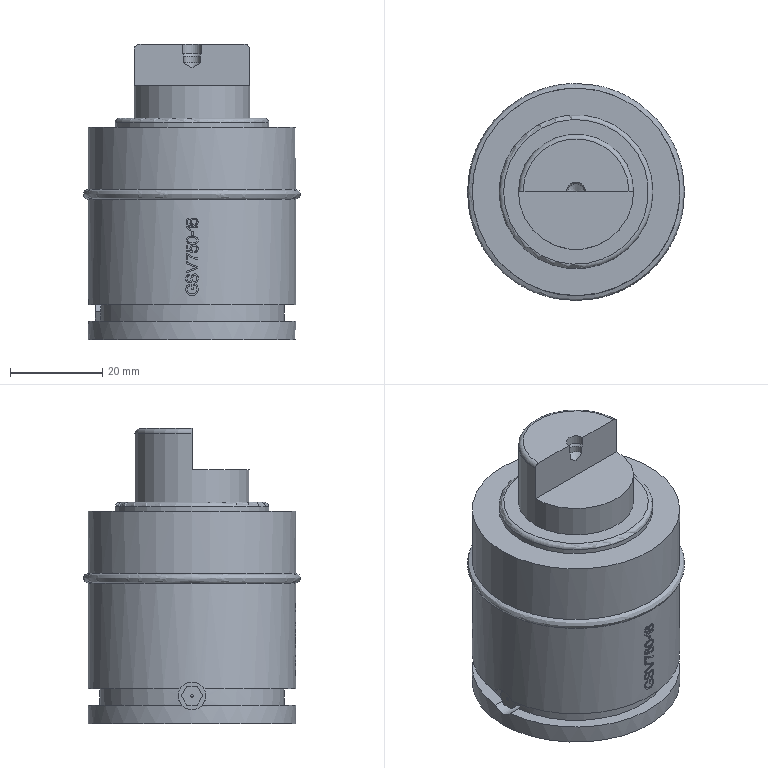Part | NX | features solid 2 | 1 solid | 165 faces | box 47.1 x 47.1 x 64 mm | volume 78740 mm3 | plane 88 | cylinder 68 | cone 6 | torus 2 | spline 1 | commonest cylinder face diameters 44.8 x9 45 x5 6.8 x2 8 x2 0.6 x1 0.72 x1